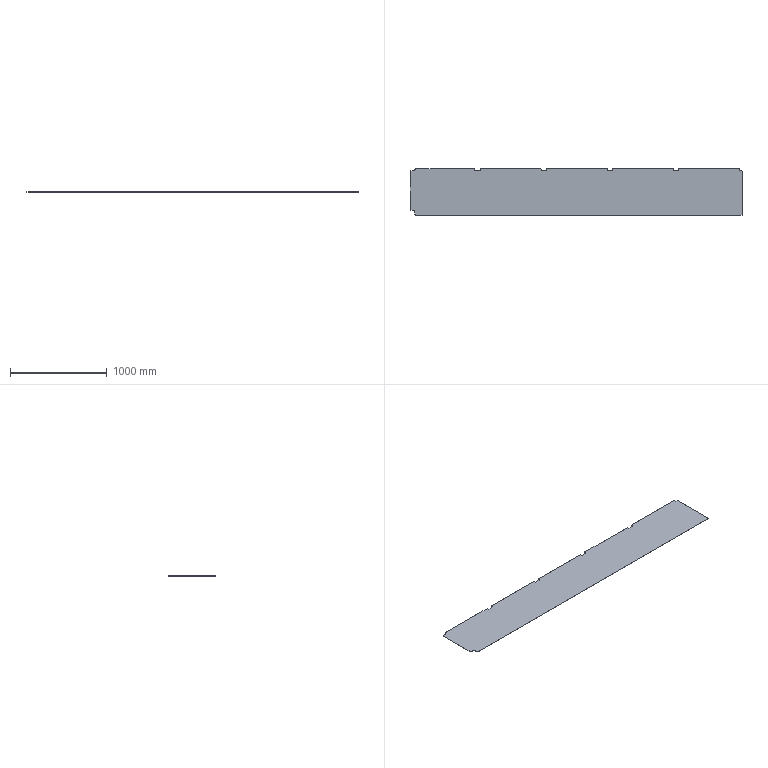Part | SolidWorks | features Cut 2, Fillet 2, FlatPattern 1, ICE 1, SMBaseFlange 1, SheetMetal 1 | 1 solid | 52 faces | box 3434 x 480 x 1.2 mm | volume 1967250 mm3 | plane 27 | cylinder 25 | commonest cylinder face diameters 6 x19 20 x6